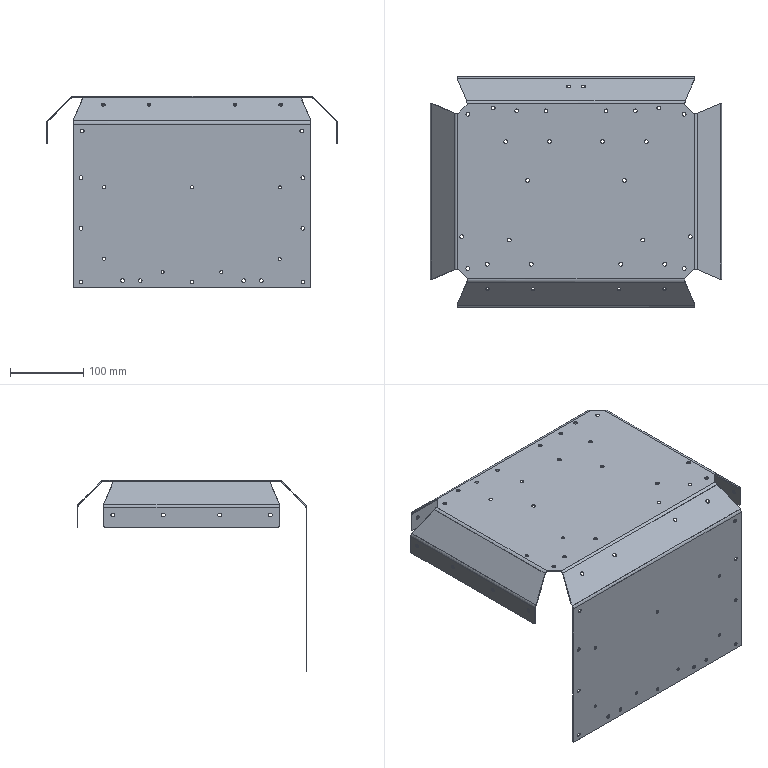Part | SolidWorks | features BaseBody 1 | 1 solid | 206 faces | box 397.6 x 313.776 x 260.905 mm | volume 271567 mm3 | cylinder 152 | plane 50 | spline 4 | commonest cylinder face diameters 5.2 x108 4.2 x14 10 x8 12.4 x8 4 x6 4.9 x6